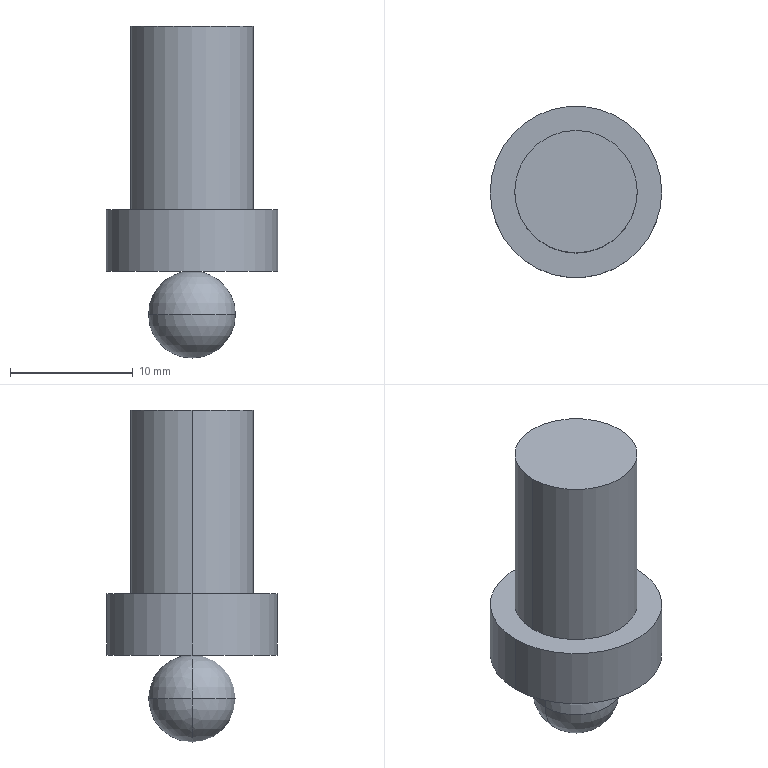Part | NX | features BREP 2 | 2 solids | 11 faces | box 14 x 14 x 27.097 mm | volume 2135 mm3 | sphere 4 | cylinder 4 | plane 3 | commonest cylinder face diameters 10 x2 14 x2
STEP:
#1=CARTESIAN_POINT('',(0.,3.548,-3.548));
#2=VERTEX_POINT('',#1);
#3=CARTESIAN_POINT('',(3.548,0.,-3.548));
#4=VERTEX_POINT('',#3);
#5=CARTESIAN_POINT('',(0.,0.,-3.548));
#6=DIRECTION('',(0.,0.,-1.));
#7=DIRECTION('',(0.,1.,0.));
#8=AXIS2_PLACEMENT_3D('',#5,#6,#7);
#9=CIRCLE('',#8,3.548);
#10=EDGE_CURVE('',#2,#4,#9,.T.);
#11=ORIENTED_EDGE('',*,*,#10,.F.);
#12=CARTESIAN_POINT('',(-3.548,0.,-3.548));
#13=VERTEX_POINT('',#12);
#14=CARTESIAN_POINT('',(0.,0.,-3.548));
#15=DIRECTION('',(0.,0.,1.));
#16=DIRECTION('',(1.,0.,0.));
#17=AXIS2_PLACEMENT_3D('',#14,#15,#16);
#18=CIRCLE('',#17,3.548);
#19=EDGE_CURVE('',#2,#13,#18,.T.);
#20=ORIENTED_EDGE('',*,*,#19,.T.);
#21=CARTESIAN_POINT('',(0.,0.,-3.548));
#22=DIRECTION('',(0.,1.,0.));
#23=DIRECTION('',(0.,0.,1.));
#24=AXIS2_PLACEMENT_3D('',#21,#22,#23);
#25=CIRCLE('',#24,3.548);
#26=EDGE_CURVE('',#13,#4,#25,.T.);
#27=ORIENTED_EDGE('',*,*,#26,.T.);
#28=EDGE_LOOP('',(#11,#20,#27));
#29=FACE_BOUND('',#28,.T.);
#30=CARTESIAN_POINT('',(0.,0.,-3.548));
#31=DIRECTION('',(0.,0.,1.));
#32=DIRECTION('',(-1.,0.,0.));
#33=AXIS2_PLACEMENT_3D('',#30,#31,#32);
#34=SPHERICAL_SURFACE('',#33,3.548);
#35=ADVANCED_FACE('',(#29),#34,.T.);
#36=ORIENTED_EDGE('',*,*,#26,.F.);
#37=CARTESIAN_POINT('',(0.,-3.548,-3.548));
#38=VERTEX_POINT('',#37);
#39=CARTESIAN_POINT('',(0.,0.,-3.548));
#40=DIRECTION('',(0.,0.,1.));
#41=DIRECTION('',(1.,0.,0.));
#42=AXIS2_PLACEMENT_3D('',#39,#40,#41);
#43=CIRCLE('',#42,3.548);
#44=EDGE_CURVE('',#13,#38,#43,.T.);
#45=ORIENTED_EDGE('',*,*,#44,.T.);
#46=CARTESIAN_POINT('',(0.,0.,-3.548));
#47=DIRECTION('',(0.,0.,-1.));
#48=DIRECTION('',(0.,1.,0.));
#49=AXIS2_PLACEMENT_3D('',#46,#47,#48);
#50=CIRCLE('',#49,3.548);
#51=EDGE_CURVE('',#4,#38,#50,.T.);
#52=ORIENTED_EDGE('',*,*,#51,.F.);
#53=EDGE_LOOP('',(#36,#45,#52));
#54=FACE_BOUND('',#53,.T.);
#55=CARTESIAN_POINT('',(0.,0.,-3.548));
#56=DIRECTION('',(0.,0.,1.));
#57=DIRECTION('',(-1.,0.,0.));
#58=AXIS2_PLACEMENT_3D('',#55,#56,#57);
#59=SPHERICAL_SURFACE('',#58,3.548);
#60=ADVANCED_FACE('',(#54),#59,.T.);
#61=ORIENTED_EDGE('',*,*,#44,.F.);
#62=CARTESIAN_POINT('',(0.,0.,-3.548));
#63=DIRECTION('',(0.,1.,0.));
#64=DIRECTION('',(0.,0.,1.));
#65=AXIS2_PLACEMENT_3D('',#62,#63,#64);
#66=CIRCLE('',#65,3.548);
#67=EDGE_CURVE('',#4,#13,#66,.T.);
#68=ORIENTED_EDGE('',*,*,#67,.F.);
#69=ORIENTED_EDGE('',*,*,#51,.T.);
#70=EDGE_LOOP('',(#61,#68,#69));
#71=FACE_BOUND('',#70,.T.);
#72=CARTESIAN_POINT('',(0.,0.,-3.548));
#73=DIRECTION('',(0.,0.,1.));
#74=DIRECTION('',(-1.,0.,0.));
#75=AXIS2_PLACEMENT_3D('',#72,#73,#74);
#76=SPHERICAL_SURFACE('',#75,3.548);
#77=ADVANCED_FACE('',(#71),#76,.T.);
#78=ORIENTED_EDGE('',*,*,#19,.F.);
#79=ORIENTED_EDGE('',*,*,#10,.T.);
#80=ORIENTED_EDGE('',*,*,#67,.T.);
#81=EDGE_LOOP('',(#78,#79,#80));
#82=FACE_BOUND('',#81,.T.);
#83=CARTESIAN_POINT('',(0.,0.,-3.548));
#84=DIRECTION('',(0.,0.,1.));
#85=DIRECTION('',(-1.,0.,0.));
#86=AXIS2_PLACEMENT_3D('',#83,#84,#85);
#87=SPHERICAL_SURFACE('',#86,3.548);
#88=ADVANCED_FACE('',(#82),#87,.T.);
#89=CLOSED_SHELL('',(#35,#60,#77,#88));
#90=MANIFOLD_SOLID_BREP('',#89);
#91=CARTESIAN_POINT('',(5.,0.,20.));
#92=VERTEX_POINT('',#91);
#93=CARTESIAN_POINT('',(-5.,0.,20.));
#94=VERTEX_POINT('',#93);
#95=CARTESIAN_POINT('',(0.,0.,20.));
#96=DIRECTION('',(0.,0.,1.));
#97=DIRECTION('',(1.,0.,0.));
#98=AXIS2_PLACEMENT_3D('',#95,#96,#97);
#99=CIRCLE('',#98,5.);
#100=EDGE_CURVE('',#92,#94,#99,.T.);
#101=ORIENTED_EDGE('',*,*,#100,.F.);
#102=CARTESIAN_POINT('',(5.,0.,5.));
#103=VERTEX_POINT('',#102);
#104=CARTESIAN_POINT('',(5.,0.,20.));
#105=DIRECTION('',(0.,0.,-1.));
#106=VECTOR('',#105,1000.);
#107=LINE('',#104,#106);
#108=EDGE_CURVE('',#103,#92,#107,.F.);
#109=ORIENTED_EDGE('',*,*,#108,.F.);
#110=CARTESIAN_POINT('',(-5.,0.,5.));
#111=VERTEX_POINT('',#110);
#112=CARTESIAN_POINT('',(0.,0.,5.));
#113=DIRECTION('',(0.,0.,1.));
#114=DIRECTION('',(1.,0.,0.));
#115=AXIS2_PLACEMENT_3D('',#112,#113,#114);
#116=CIRCLE('',#115,5.);
#117=EDGE_CURVE('',#103,#111,#116,.T.);
#118=ORIENTED_EDGE('',*,*,#117,.T.);
#119=CARTESIAN_POINT('',(-5.,0.,20.));
#120=DIRECTION('',(0.,0.,-1.));
#121=VECTOR('',#120,1000.);
#122=LINE('',#119,#121);
#123=EDGE_CURVE('',#111,#94,#122,.F.);
#124=ORIENTED_EDGE('',*,*,#123,.T.);
#125=EDGE_LOOP('',(#101,#109,#118,#124));
#126=FACE_BOUND('',#125,.T.);
#127=CARTESIAN_POINT('',(0.,0.,20.));
#128=DIRECTION('',(0.,0.,-1.));
#129=DIRECTION('',(1.,0.,0.));
#130=AXIS2_PLACEMENT_3D('',#127,#128,#129);
#131=CYLINDRICAL_SURFACE('',#130,5.);
#132=ADVANCED_FACE('',(#126),#131,.T.);
#133=CARTESIAN_POINT('',(7.,0.,5.));
#134=VERTEX_POINT('',#133);
#135=CARTESIAN_POINT('',(-7.,0.,5.));
#136=VERTEX_POINT('',#135);
#137=CARTESIAN_POINT('',(0.,0.,5.));
#138=DIRECTION('',(0.,0.,1.));
#139=DIRECTION('',(1.,0.,0.));
#140=AXIS2_PLACEMENT_3D('',#137,#138,#139);
#141=CIRCLE('',#140,7.);
#142=EDGE_CURVE('',#134,#136,#141,.T.);
#143=ORIENTED_EDGE('',*,*,#142,.F.);
#144=CARTESIAN_POINT('',(7.,0.,0.));
#145=VERTEX_POINT('',#144);
#146=CARTESIAN_POINT('',(7.,0.,5.));
#147=DIRECTION('',(0.,0.,-1.));
#148=VECTOR('',#147,1000.);
#149=LINE('',#146,#148);
#150=EDGE_CURVE('',#145,#134,#149,.F.);
#151=ORIENTED_EDGE('',*,*,#150,.F.);
#152=CARTESIAN_POINT('',(-7.,0.,0.));
#153=VERTEX_POINT('',#152);
#154=CARTESIAN_POINT('',(0.,0.,0.));
#155=DIRECTION('',(0.,0.,1.));
#156=DIRECTION('',(1.,0.,0.));
#157=AXIS2_PLACEMENT_3D('',#154,#155,#156);
#158=CIRCLE('',#157,7.);
#159=EDGE_CURVE('',#145,#153,#158,.T.);
#160=ORIENTED_EDGE('',*,*,#159,.T.);
#161=CARTESIAN_POINT('',(-7.,0.,5.));
#162=DIRECTION('',(0.,0.,-1.));
#163=VECTOR('',#162,1000.);
#164=LINE('',#161,#163);
#165=EDGE_CURVE('',#153,#136,#164,.F.);
#166=ORIENTED_EDGE('',*,*,#165,.T.);
#167=EDGE_LOOP('',(#143,#151,#160,#166));
#168=FACE_BOUND('',#167,.T.);
#169=CARTESIAN_POINT('',(0.,0.,5.));
#170=DIRECTION('',(0.,0.,-1.));
#171=DIRECTION('',(1.,0.,0.));
#172=AXIS2_PLACEMENT_3D('',#169,#170,#171);
#173=CYLINDRICAL_SURFACE('',#172,7.);
#174=ADVANCED_FACE('',(#168),#173,.T.);
#175=CARTESIAN_POINT('',(0.,0.,5.));
#176=DIRECTION('',(0.,0.,1.));
#177=DIRECTION('',(1.,0.,0.));
#178=AXIS2_PLACEMENT_3D('',#175,#176,#177);
#179=CIRCLE('',#178,7.);
#180=EDGE_CURVE('',#136,#134,#179,.T.);
#181=ORIENTED_EDGE('',*,*,#180,.T.);
#182=ORIENTED_EDGE('',*,*,#142,.T.);
#183=EDGE_LOOP('',(#181,#182));
#184=FACE_BOUND('',#183,.T.);
#185=CARTESIAN_POINT('',(0.,0.,5.));
#186=DIRECTION('',(0.,0.,1.));
#187=DIRECTION('',(1.,0.,0.));
#188=AXIS2_PLACEMENT_3D('',#185,#186,#187);
#189=CIRCLE('',#188,5.);
#190=EDGE_CURVE('',#111,#103,#189,.T.);
#191=ORIENTED_EDGE('',*,*,#190,.F.);
#192=ORIENTED_EDGE('',*,*,#117,.F.);
#193=EDGE_LOOP('',(#191,#192));
#194=FACE_BOUND('',#193,.T.);
#195=CARTESIAN_POINT('',(0.,0.,5.));
#196=DIRECTION('',(0.,0.,1.));
#197=DIRECTION('',(0.,1.,0.));
#198=AXIS2_PLACEMENT_3D('',#195,#196,#197);
#199=PLANE('',#198);
#200=ADVANCED_FACE('',(#184,#194),#199,.T.);
#201=ORIENTED_EDGE('',*,*,#150,.T.);
#202=ORIENTED_EDGE('',*,*,#180,.F.);
#203=ORIENTED_EDGE('',*,*,#165,.F.);
#204=CARTESIAN_POINT('',(0.,0.,0.));
#205=DIRECTION('',(0.,0.,1.));
#206=DIRECTION('',(1.,0.,0.));
#207=AXIS2_PLACEMENT_3D('',#204,#205,#206);
#208=CIRCLE('',#207,7.);
#209=EDGE_CURVE('',#153,#145,#208,.T.);
#210=ORIENTED_EDGE('',*,*,#209,.T.);
#211=EDGE_LOOP('',(#201,#202,#203,#210));
#212=FACE_BOUND('',#211,.T.);
#213=CARTESIAN_POINT('',(0.,0.,5.));
#214=DIRECTION('',(0.,0.,-1.));
#215=DIRECTION('',(1.,0.,0.));
#216=AXIS2_PLACEMENT_3D('',#213,#214,#215);
#217=CYLINDRICAL_SURFACE('',#216,7.);
#218=ADVANCED_FACE('',(#212),#217,.T.);
#219=ORIENTED_EDGE('',*,*,#209,.F.);
#220=ORIENTED_EDGE('',*,*,#159,.F.);
#221=EDGE_LOOP('',(#219,#220));
#222=FACE_BOUND('',#221,.T.);
#223=CARTESIAN_POINT('',(0.,0.,0.));
#224=DIRECTION('',(0.,0.,1.));
#225=DIRECTION('',(0.,1.,0.));
#226=AXIS2_PLACEMENT_3D('',#223,#224,#225);
#227=PLANE('',#226);
#228=ADVANCED_FACE('',(#222),#227,.F.);
#229=ORIENTED_EDGE('',*,*,#108,.T.);
#230=CARTESIAN_POINT('',(0.,0.,20.));
#231=DIRECTION('',(0.,0.,1.));
#232=DIRECTION('',(1.,0.,0.));
#233=AXIS2_PLACEMENT_3D('',#230,#231,#232);
#234=CIRCLE('',#233,5.);
#235=EDGE_CURVE('',#94,#92,#234,.T.);
#236=ORIENTED_EDGE('',*,*,#235,.F.);
#237=ORIENTED_EDGE('',*,*,#123,.F.);
#238=ORIENTED_EDGE('',*,*,#190,.T.);
#239=EDGE_LOOP('',(#229,#236,#237,#238));
#240=FACE_BOUND('',#239,.T.);
#241=CARTESIAN_POINT('',(0.,0.,20.));
#242=DIRECTION('',(0.,0.,-1.));
#243=DIRECTION('',(1.,0.,0.));
#244=AXIS2_PLACEMENT_3D('',#241,#242,#243);
#245=CYLINDRICAL_SURFACE('',#244,5.);
#246=ADVANCED_FACE('',(#240),#245,.T.);
#247=ORIENTED_EDGE('',*,*,#235,.T.);
#248=ORIENTED_EDGE('',*,*,#100,.T.);
#249=EDGE_LOOP('',(#247,#248));
#250=FACE_BOUND('',#249,.T.);
#251=CARTESIAN_POINT('',(0.,0.,20.));
#252=DIRECTION('',(0.,0.,1.));
#253=DIRECTION('',(0.,1.,0.));
#254=AXIS2_PLACEMENT_3D('',#251,#252,#253);
#255=PLANE('',#254);
#256=ADVANCED_FACE('',(#250),#255,.T.);
#257=CLOSED_SHELL('',(#132,#174,#200,#218,#228,#246,#256));
#258=MANIFOLD_SOLID_BREP('',#257);
#259=(LENGTH_UNIT()NAMED_UNIT(*)SI_UNIT(.MILLI.,.METRE.));
#260=UNCERTAINTY_MEASURE_WITH_UNIT(LENGTH_MEASURE(0.00001),#259,'','');
#261=(NAMED_UNIT(*)PLANE_ANGLE_UNIT()SI_UNIT($,.RADIAN.));
#262=(NAMED_UNIT(*)SI_UNIT($,.STERADIAN.)SOLID_ANGLE_UNIT());
#263=(GEOMETRIC_REPRESENTATION_CONTEXT(3)GLOBAL_UNCERTAINTY_ASSIGNED_CONTEXT((#260))GLOBAL_UNIT_ASSIGNED_CONTEXT((#259,#261,#262))REPRESENTATION_CONTEXT('',''));
#264=ADVANCED_BREP_SHAPE_REPRESENTATION('',(#90,#258),#263);